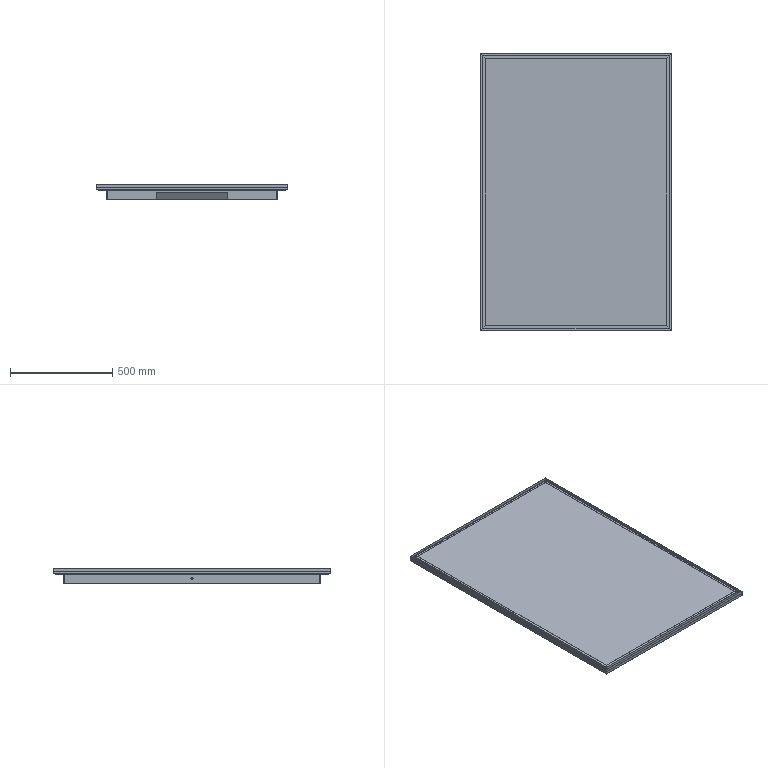Part | SolidWorks | 7 solids | 282 faces | box 940 x 1360 x 75 mm | volume 28124716 mm3 | plane 148 | cylinder 122 | spline 12 | commonest cylinder face diameters 4.2 x80 11 x14 0.4 x11 2.4 x11 10 x6